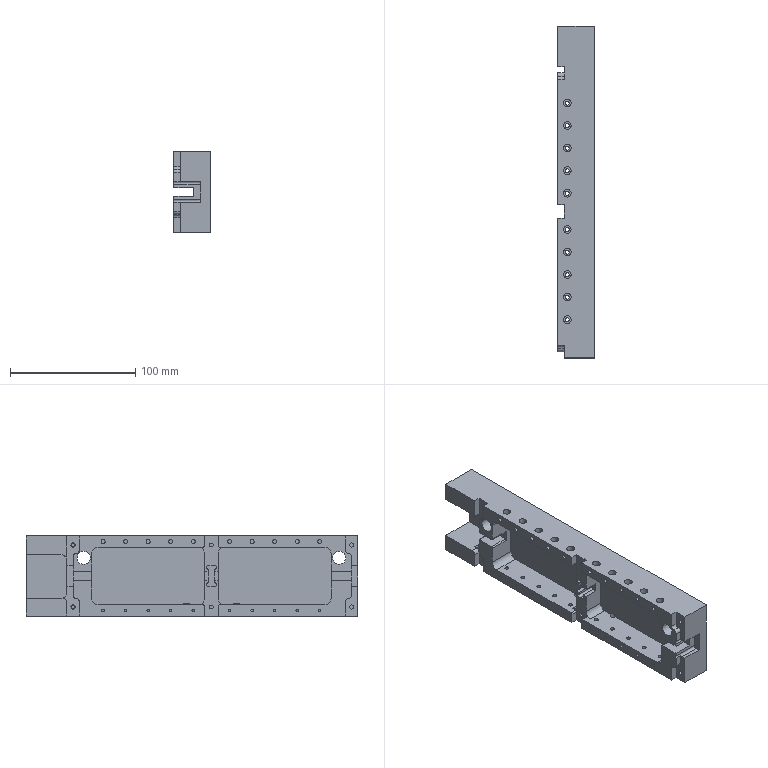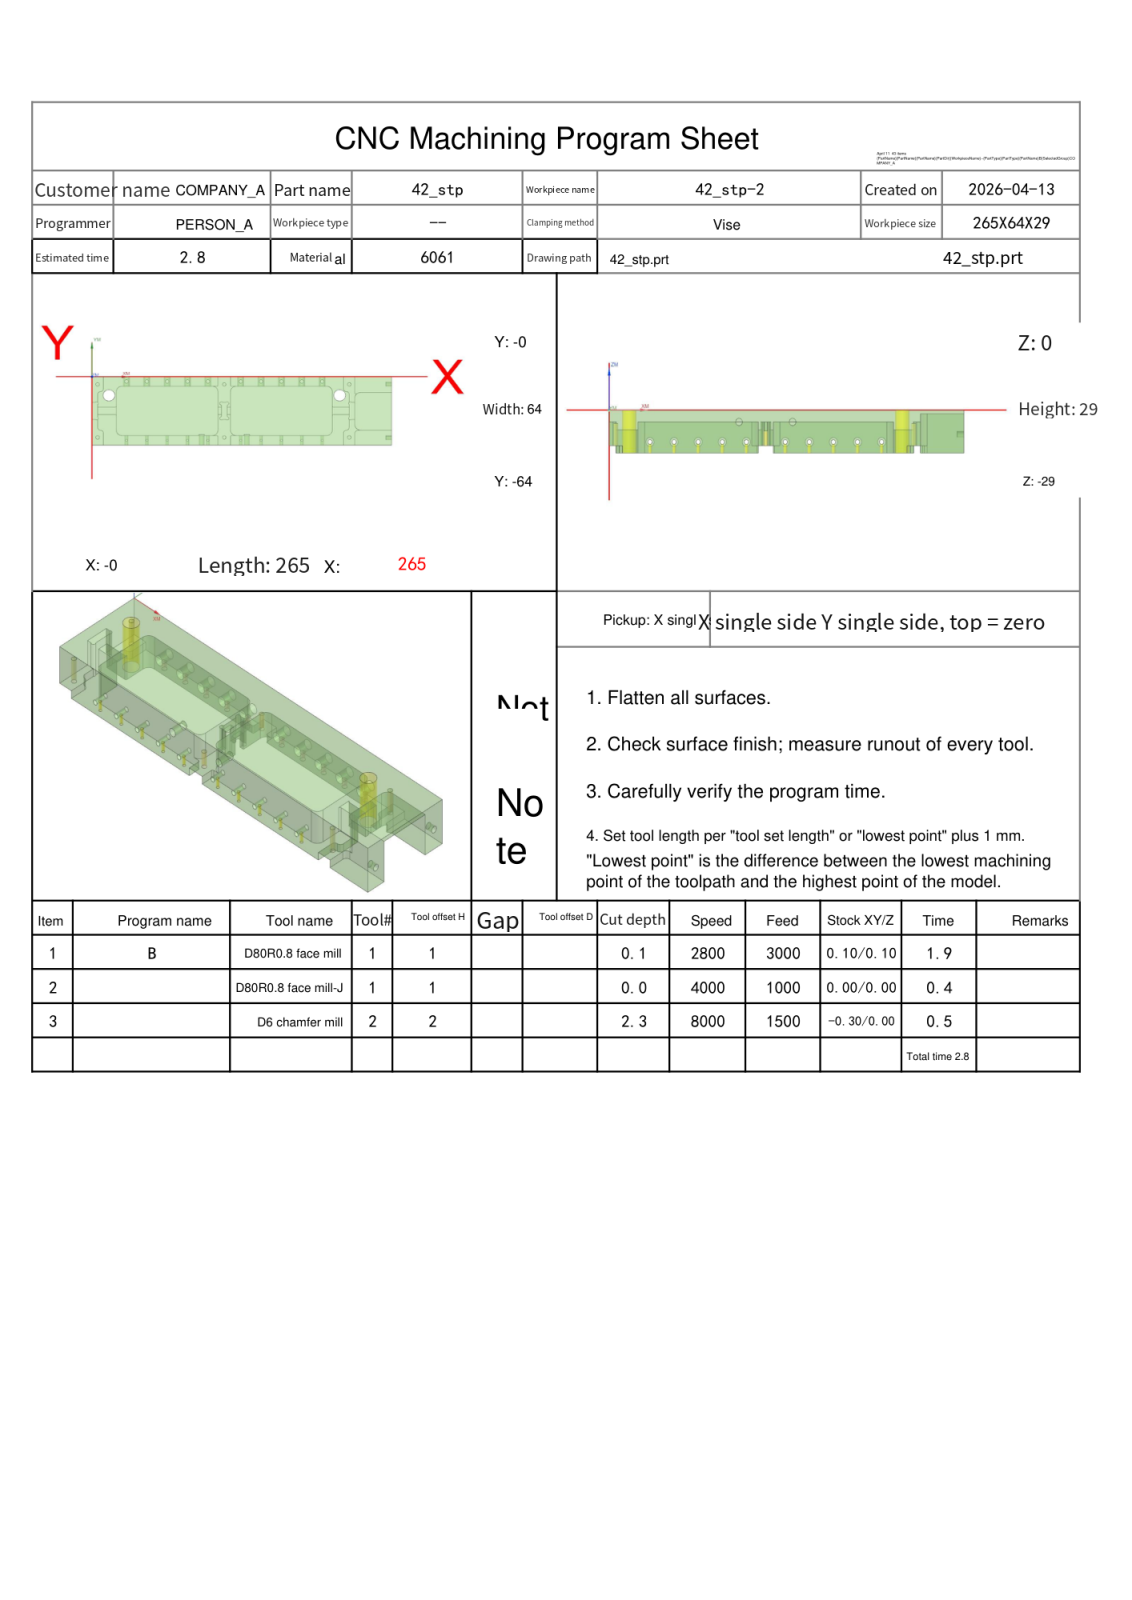NC program | NX | posted by the shop | part box 29 x 265 x 64 mm
Whole program:
%
O0001
(Machine time: 3.34 MIN)
(===Total Tool:2===)
(T1=D80R0.8 face mill D=80.  R=0.8  D-  H01 Z=0.    )
(T2=D6 chamfer mill   D=6.   R=0.   D-  H02 Z=-2.3  )
G80 G90 G17 G49 G40
G91 G28 Z0
M01
N1 T01 M06
(D80R0.8 face mill  D=80. R=0.8 H=01 ce=0.10 di=0.10)
G00 G90 G54 X-52.097 Y-32. M03 S2800
G43 H01 Z20.
M08
Z7.325
G01 Z5.325 F3000.
X-40.097
X305.097
X317.097
Z7.325
G00 X-52.097
Z6.85
G01 Z4.85
X-40.097
X305.097
X317.097
Z6.85
G00 X-52.097
Z6.375
G01 Z4.375
X-40.097
X305.097
X317.097
Z6.375
G00 X-52.097
Z5.9
G01 Z3.9
X-40.097
X305.097
X317.097
Z5.9
G00 Z20.
X-52.097
Z5.425
G01 Z3.425
X-40.097
X305.097
X317.097
Z5.425
G00 Z20.
X-52.097
Z4.95
G01 Z2.95
X-40.097
X305.097
X317.097
Z4.95
G00 Z20.
X-52.097
Z4.475
G01 Z2.475
X-40.097
X305.097
X317.097
Z4.475
G00 Z20.
X-52.097
Z4.
G01 Z2.
X-40.097
X305.097
X317.097
Z4.
G00 Z20.
X-52.097
Z3.525
G01 Z1.525
X-40.097
X305.097
X317.097
Z3.525
G00 Z20.
X-52.097
Z3.05
G01 Z1.05
X-40.097
X305.097
X317.097
Z3.05
G00 Z20.
X-52.097
Z2.575
G01 Z.575
X-40.097
X305.097
X317.097
Z2.575
G00 Z20.
X-52.097
Z2.1
G01 Z.1
X-40.097
X305.097
X317.097
Z2.1
G00 Z20.
G91 G28 Z0.0
M05
M09
G91 G28 Z0.0
M01
N2 T01 M06
(D80R0.8 face mill-J  D=80. R=0.8 H=01 ce=0.00 di=0.00)
G00 G90 G54 X-51.999 Y-32. M03 S4000
G43 H01 Z20.
M08
Z2.
G01 Z0.0 F1000.
X-39.999
X304.999
X316.999
Z2.
G00 Z20.
G91 G28 Z0.0
M05
M09
G91 G28 Z0.0
M01
N3 T02 M06
(D6 chamfer mill  D=6. R=0. H=02 ce=-0.30 di=0.00)
G00 G90 G54 X221.242 Y-17.313 M03 S8000
G43 H02 Z20.
M08
Z-1.8
G01 Z-2.3 F1200.
X222. Y-17.25
G03 X219. Y-14.25 I-3. J0.0
X215.75 Y-17.5 I0.0 J-3.25
X219. Y-20.75 I3.25 J0.0
X222.25 Y-17.5 I0.0 J3.25
X219. Y-14.25 I-3.25 J0.0
X216. Y-17.25 I0.0 J-3.
G01 X216.758 Y-17.313
Z-1.8
G00 Z20.
X12.758 Y-17.687
Z-1.8
G01 Z-2.3
X12. Y-17.75
G03 X15. Y-20.75 I3. J0.0
X18.25 Y-17.5 I0.0 J3.25
X15. Y-14.25 I-3.25 J0.0
X11.75 Y-17.5 I0.0 J-3.25
X15. Y-20.75 I3.25 J0.0
X18. Y-17.75 I0.0 J3.
G01 X17.242 Y-17.687
Z-1.8
G00 Z20.
G00 G90 X265.7 Y-55.657 M03 S7000
Z20.
Z2.5
G01 Y-63.7 Z-.428 F1500.
Y-63.778 Z-.456
X265.664 Y-63.977 Z-.529
X265.589 Y-64.165 Z-.603
X265.477 Y-64.334 Z-.677
X265.334 Y-64.477 Z-.751
X265.165 Y-64.589 Z-.824
X264.977 Y-64.664 Z-.898
X264.778 Y-64.7 Z-.972
X264.7 Z-1.
X.3
G02 X-.7 Y-63.7 I0.0 J1.
G01 Y-.3
G02 X.3 Y.7 I1. J0.0
G01 X264.7
G02 X265.7 Y-.3 I0.0 J-1.
G01 Y-63.7
G02 X264.7 Y-64.7 I-1. J0.0
G01 X264.2
Z1.5
G00 Z20.
M05
M09
G91 G28 Z0.0
G91 G28 Y0.0
M30
%